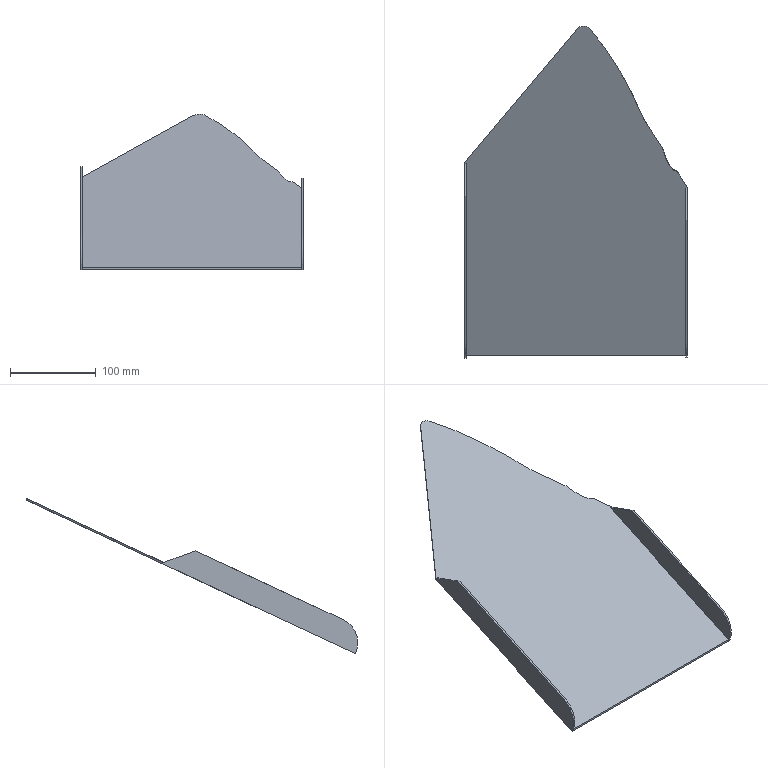Part | NX | features solid 2 | 1 solid | 18 faces | box 260.45 x 387.608 x 181.641 mm | volume 198390 mm3 | plane 12 | spline 3 | cylinder 3 | commonest cylinder face diameters 60 x2 20 x1
STEP:
#1=CARTESIAN_POINT('',(-285.45,-615.955,-192.902));
#2=VERTEX_POINT('',#1);
#3=CARTESIAN_POINT('',(-283.45,-615.955,-192.902));
#4=VERTEX_POINT('',#3);
#5=CARTESIAN_POINT('',(-285.45,-615.955,-192.902));
#6=DIRECTION('',(-1.,0.,0.));
#7=VECTOR('',#6,1000.);
#8=LINE('',#5,#7);
#9=EDGE_CURVE('',#2,#4,#8,.F.);
#10=ORIENTED_EDGE('',*,*,#9,.T.);
#11=CARTESIAN_POINT('',(-283.45,-840.,-297.376));
#12=VERTEX_POINT('',#11);
#13=CARTESIAN_POINT('',(-283.45,-651.161,-209.318));
#14=DIRECTION('',(0.,-0.9063,-0.4226));
#15=VECTOR('',#14,1000.);
#16=LINE('',#13,#15);
#17=EDGE_CURVE('',#4,#12,#16,.T.);
#18=ORIENTED_EDGE('',*,*,#17,.T.);
#19=CARTESIAN_POINT('',(-27.,-840.,-297.376));
#20=VERTEX_POINT('',#19);
#21=CARTESIAN_POINT('',(-1209.175,-840.,-297.376));
#22=DIRECTION('',(-1.,0.,0.));
#23=VECTOR('',#22,1000.);
#24=LINE('',#21,#23);
#25=EDGE_CURVE('',#12,#20,#24,.F.);
#26=ORIENTED_EDGE('',*,*,#25,.T.);
#27=CARTESIAN_POINT('',(-27.,-644.804,-206.354));
#28=VERTEX_POINT('',#27);
#29=CARTESIAN_POINT('',(-27.,-651.161,-209.318));
#30=DIRECTION('',(0.,-0.9063,-0.4226));
#31=VECTOR('',#30,1000.);
#32=LINE('',#29,#31);
#33=EDGE_CURVE('',#28,#20,#32,.T.);
#34=ORIENTED_EDGE('',*,*,#33,.F.);
#35=CARTESIAN_POINT('',(-25.,-644.804,-206.354));
#36=VERTEX_POINT('',#35);
#37=CARTESIAN_POINT('',(-25.,-644.804,-206.354));
#38=DIRECTION('',(1.,0.,0.));
#39=VECTOR('',#38,1000.);
#40=LINE('',#37,#39);
#41=EDGE_CURVE('',#28,#36,#40,.T.);
#42=ORIENTED_EDGE('',*,*,#41,.T.);
#43=CARTESIAN_POINT('',(-25.,-643.958,-205.96));
#44=VERTEX_POINT('',#43);
#45=CARTESIAN_POINT('',(-25.,-651.161,-209.318));
#46=DIRECTION('',(0.,-0.9063,-0.4226));
#47=VECTOR('',#46,1000.);
#48=LINE('',#45,#47);
#49=EDGE_CURVE('',#44,#36,#48,.T.);
#50=ORIENTED_EDGE('',*,*,#49,.F.);
#51=CARTESIAN_POINT('',(-36.874,-625.397,-197.305));
#52=VERTEX_POINT('',#51);
#53=CARTESIAN_POINT('',(-25.,-643.958,-205.96));
#54=CARTESIAN_POINT('',(-28.958,-637.771,-203.075));
#55=CARTESIAN_POINT('',(-32.916,-631.584,-200.19));
#56=CARTESIAN_POINT('',(-36.874,-625.397,-197.305));
#57=B_SPLINE_CURVE_WITH_KNOTS('',3,(#53,#54,#55,#56),.UNSPECIFIED.,.F.,.F.,(4,4),(0.,0.02367),.UNSPECIFIED.);
#58=EDGE_CURVE('',#44,#52,#57,.T.);
#59=ORIENTED_EDGE('',*,*,#58,.T.);
#60=CARTESIAN_POINT('',(-53.995,-598.635,-184.825));
#61=VERTEX_POINT('',#60);
#62=CARTESIAN_POINT('',(-36.874,-625.397,-197.305));
#63=CARTESIAN_POINT('',(-39.726,-624.678,-196.969));
#64=CARTESIAN_POINT('',(-44.629,-621.228,-195.361));
#65=CARTESIAN_POINT('',(-48.688,-613.987,-191.984));
#66=CARTESIAN_POINT('',(-51.509,-606.353,-188.424));
#67=CARTESIAN_POINT('',(-53.147,-601.203,-186.022));
#68=CARTESIAN_POINT('',(-53.995,-598.635,-184.825));
#69=B_SPLINE_CURVE_WITH_KNOTS('',3,(#62,#63,#64,#65,#66,#67,#68),.UNSPECIFIED.,.F.,.F.,(4,1,1,1,4),(0.0119,0.0208,0.0297,0.0386,0.0475),.UNSPECIFIED.);
#70=EDGE_CURVE('',#52,#61,#69,.T.);
#71=ORIENTED_EDGE('',*,*,#70,.T.);
#72=CARTESIAN_POINT('',(-139.243,-458.439,-119.451));
#73=VERTEX_POINT('',#72);
#74=CARTESIAN_POINT('',(-53.995,-598.635,-184.825));
#75=CARTESIAN_POINT('',(-55.837,-595.756,-183.483));
#76=CARTESIAN_POINT('',(-59.52,-589.999,-180.798));
#77=CARTESIAN_POINT('',(-65.043,-581.362,-176.77));
#78=CARTESIAN_POINT('',(-69.653,-574.168,-173.416));
#79=CARTESIAN_POINT('',(-72.866,-569.125,-171.064));
#80=CARTESIAN_POINT('',(-74.724,-566.254,-169.726));
#81=CARTESIAN_POINT('',(-76.066,-564.075,-168.71));
#82=CARTESIAN_POINT('',(-77.109,-561.743,-167.622));
#83=CARTESIAN_POINT('',(-78.457,-559.567,-166.607));
#84=CARTESIAN_POINT('',(-79.554,-557.262,-165.533));
#85=CARTESIAN_POINT('',(-80.855,-554.106,-164.061));
#86=CARTESIAN_POINT('',(-82.504,-550.172,-162.227));
#87=CARTESIAN_POINT('',(-86.598,-540.797,-157.855));
#88=CARTESIAN_POINT('',(-93.303,-527.007,-151.425));
#89=CARTESIAN_POINT('',(-103.21,-509.091,-143.07));
#90=CARTESIAN_POINT('',(-114.016,-491.603,-134.915));
#91=CARTESIAN_POINT('',(-125.687,-474.559,-126.967));
#92=CARTESIAN_POINT('',(-134.482,-463.624,-121.868));
#93=CARTESIAN_POINT('',(-139.243,-458.439,-119.451));
#94=B_SPLINE_CURVE_WITH_KNOTS('',3,(#74,#75,#76,#77,#78,#79,#80,#81,#82,#83,#84,#85,#86,#87,#88,#89,#90,#91,#92,#93),.UNSPECIFIED.,.F.,.F.,(4,1,1,1,1,1,1,1,1,1,1,1,1,1,1,1,1,4),(0.0578,0.06882,0.07983,0.09085,0.09635,0.09911,0.1019,0.1046,0.1074,0.1101,0.1129,0.1184,0.1239,0.1459,0.1679,0.19,0.212,0.234),.UNSPECIFIED.);
#95=EDGE_CURVE('',#61,#73,#94,.T.);
#96=ORIENTED_EDGE('',*,*,#95,.T.);
#97=CARTESIAN_POINT('',(-154.269,-458.775,-119.607));
#98=VERTEX_POINT('',#97);
#99=CARTESIAN_POINT('',(-146.609,-465.203,-122.605));
#100=DIRECTION('',(0.,-0.4226,0.9063));
#101=DIRECTION('',(0.,-0.9063,-0.4226));
#102=AXIS2_PLACEMENT_3D('',#99,#100,#101);
#103=ELLIPSE('',#102,11.034,10.);
#104=EDGE_CURVE('',#73,#98,#103,.T.);
#105=ORIENTED_EDGE('',*,*,#104,.T.);
#106=CARTESIAN_POINT('',(-285.45,-615.11,-192.507));
#107=VERTEX_POINT('',#106);
#108=CARTESIAN_POINT('',(-643.087,-1041.326,-391.255));
#109=DIRECTION('',(0.6053,0.7214,0.3364));
#110=VECTOR('',#109,1000.);
#111=LINE('',#108,#110);
#112=EDGE_CURVE('',#107,#98,#111,.T.);
#113=ORIENTED_EDGE('',*,*,#112,.F.);
#114=CARTESIAN_POINT('',(-285.45,-651.161,-209.318));
#115=DIRECTION('',(0.,-0.9063,-0.4226));
#116=VECTOR('',#115,1000.);
#117=LINE('',#114,#116);
#118=EDGE_CURVE('',#107,#2,#117,.T.);
#119=ORIENTED_EDGE('',*,*,#118,.T.);
#120=EDGE_LOOP('',(#10,#18,#26,#34,#42,#50,#59,#71,#96,#105,#113,#119));
#121=FACE_BOUND('',#120,.T.);
#122=CARTESIAN_POINT('',(-1209.175,-651.161,-209.318));
#123=DIRECTION('',(0.,-0.4226,0.9063));
#124=DIRECTION('',(1.,0.,0.));
#125=AXIS2_PLACEMENT_3D('',#122,#123,#124);
#126=PLANE('',#125);
#127=ADVANCED_FACE('',(#121),#126,.T.);
#128=ORIENTED_EDGE('',*,*,#25,.F.);
#129=CARTESIAN_POINT('',(-283.45,-840.,-299.582));
#130=VERTEX_POINT('',#129);
#131=CARTESIAN_POINT('',(-283.45,-840.,-720.));
#132=DIRECTION('',(0.,0.,1.));
#133=VECTOR('',#132,1000.);
#134=LINE('',#131,#133);
#135=EDGE_CURVE('',#12,#130,#134,.F.);
#136=ORIENTED_EDGE('',*,*,#135,.T.);
#137=CARTESIAN_POINT('',(-27.,-840.,-299.582));
#138=VERTEX_POINT('',#137);
#139=CARTESIAN_POINT('',(-1209.175,-840.,-299.582));
#140=DIRECTION('',(-1.,0.,0.));
#141=VECTOR('',#140,1000.);
#142=LINE('',#139,#141);
#143=EDGE_CURVE('',#130,#138,#142,.F.);
#144=ORIENTED_EDGE('',*,*,#143,.T.);
#145=CARTESIAN_POINT('',(-27.,-840.,-720.));
#146=DIRECTION('',(0.,0.,1.));
#147=VECTOR('',#146,1000.);
#148=LINE('',#145,#147);
#149=EDGE_CURVE('',#20,#138,#148,.F.);
#150=ORIENTED_EDGE('',*,*,#149,.F.);
#151=EDGE_LOOP('',(#128,#136,#144,#150));
#152=FACE_BOUND('',#151,.T.);
#153=CARTESIAN_POINT('',(-476.248,-840.,-720.));
#154=DIRECTION('',(0.,1.,0.));
#155=DIRECTION('',(-1.,0.,0.));
#156=AXIS2_PLACEMENT_3D('',#153,#154,#155);
#157=PLANE('',#156);
#158=ADVANCED_FACE('',(#152),#157,.F.);
#159=CARTESIAN_POINT('',(-285.45,-615.11,-194.714));
#160=VERTEX_POINT('',#159);
#161=CARTESIAN_POINT('',(-285.45,-840.,-299.582));
#162=VERTEX_POINT('',#161);
#163=CARTESIAN_POINT('',(-285.45,-650.315,-211.131));
#164=DIRECTION('',(0.,-0.9063,-0.4226));
#165=VECTOR('',#164,1000.);
#166=LINE('',#163,#165);
#167=EDGE_CURVE('',#160,#162,#166,.T.);
#168=ORIENTED_EDGE('',*,*,#167,.F.);
#169=CARTESIAN_POINT('',(-154.269,-458.775,-121.814));
#170=VERTEX_POINT('',#169);
#171=CARTESIAN_POINT('',(-642.638,-1040.79,-393.212));
#172=DIRECTION('',(0.6053,0.7214,0.3364));
#173=VECTOR('',#172,1000.);
#174=LINE('',#171,#173);
#175=EDGE_CURVE('',#160,#170,#174,.T.);
#176=ORIENTED_EDGE('',*,*,#175,.T.);
#177=CARTESIAN_POINT('',(-139.243,-458.439,-121.657));
#178=VERTEX_POINT('',#177);
#179=CARTESIAN_POINT('',(-146.609,-465.203,-124.811));
#180=DIRECTION('',(0.,-0.4226,0.9063));
#181=DIRECTION('',(0.,-0.9063,-0.4226));
#182=AXIS2_PLACEMENT_3D('',#179,#180,#181);
#183=ELLIPSE('',#182,11.034,10.);
#184=EDGE_CURVE('',#170,#178,#183,.F.);
#185=ORIENTED_EDGE('',*,*,#184,.T.);
#186=CARTESIAN_POINT('',(-53.417,-599.538,-187.453));
#187=VERTEX_POINT('',#186);
#188=CARTESIAN_POINT('',(-53.417,-599.538,-187.453));
#189=CARTESIAN_POINT('',(-55.271,-596.64,-186.102));
#190=CARTESIAN_POINT('',(-58.978,-590.845,-183.399));
#191=CARTESIAN_POINT('',(-64.541,-582.153,-179.346));
#192=CARTESIAN_POINT('',(-69.169,-574.906,-175.967));
#193=CARTESIAN_POINT('',(-72.423,-569.841,-173.605));
#194=CARTESIAN_POINT('',(-74.261,-566.935,-172.25));
#195=CARTESIAN_POINT('',(-75.7,-564.787,-171.248));
#196=CARTESIAN_POINT('',(-76.761,-562.445,-170.156));
#197=CARTESIAN_POINT('',(-78.054,-560.222,-169.12));
#198=CARTESIAN_POINT('',(-79.26,-557.954,-168.062));
#199=CARTESIAN_POINT('',(-80.578,-554.782,-166.583));
#200=CARTESIAN_POINT('',(-82.227,-550.817,-164.734));
#201=CARTESIAN_POINT('',(-86.333,-541.374,-160.331));
#202=CARTESIAN_POINT('',(-93.051,-527.479,-153.852));
#203=CARTESIAN_POINT('',(-103.006,-509.438,-145.439));
#204=CARTESIAN_POINT('',(-113.867,-491.828,-137.227));
#205=CARTESIAN_POINT('',(-125.604,-474.667,-129.225));
#206=CARTESIAN_POINT('',(-134.451,-463.657,-124.091));
#207=CARTESIAN_POINT('',(-139.243,-458.439,-121.657));
#208=B_SPLINE_CURVE_WITH_KNOTS('',3,(#188,#189,#190,#191,#192,#193,#194,#195,#196,#197,#198,#199,#200,#201,#202,#203,#204,#205,#206,#207),.UNSPECIFIED.,.F.,.F.,(4,1,1,1,1,1,1,1,1,1,1,1,1,1,1,1,1,4),(0.05665,0.06774,0.07882,0.08991,0.09545,0.09823,0.101,0.1038,0.1065,0.1093,0.1121,0.1176,0.1232,0.1453,0.1675,0.1897,0.2119,0.234),.UNSPECIFIED.);
#209=EDGE_CURVE('',#187,#178,#208,.T.);
#210=ORIENTED_EDGE('',*,*,#209,.F.);
#211=CARTESIAN_POINT('',(-37.534,-624.366,-199.031));
#212=VERTEX_POINT('',#211);
#213=CARTESIAN_POINT('',(-37.534,-624.366,-199.031));
#214=CARTESIAN_POINT('',(-40.104,-623.568,-198.658));
#215=CARTESIAN_POINT('',(-44.555,-620.328,-197.148));
#216=CARTESIAN_POINT('',(-48.394,-613.718,-194.065));
#217=CARTESIAN_POINT('',(-51.125,-606.69,-190.788));
#218=CARTESIAN_POINT('',(-52.632,-601.916,-188.562));
#219=CARTESIAN_POINT('',(-53.417,-599.538,-187.453));
#220=B_SPLINE_CURVE_WITH_KNOTS('',3,(#213,#214,#215,#216,#217,#218,#219),.UNSPECIFIED.,.F.,.F.,(4,1,1,1,4),(0.0126,0.02081,0.02901,0.03722,0.04543),.UNSPECIFIED.);
#221=EDGE_CURVE('',#212,#187,#220,.T.);
#222=ORIENTED_EDGE('',*,*,#221,.F.);
#223=CARTESIAN_POINT('',(-25.,-643.958,-208.167));
#224=VERTEX_POINT('',#223);
#225=CARTESIAN_POINT('',(-25.,-643.958,-208.167));
#226=CARTESIAN_POINT('',(-29.178,-637.428,-205.121));
#227=CARTESIAN_POINT('',(-33.356,-630.897,-202.076));
#228=CARTESIAN_POINT('',(-37.534,-624.366,-199.031));
#229=B_SPLINE_CURVE_WITH_KNOTS('',3,(#225,#226,#227,#228),.UNSPECIFIED.,.F.,.F.,(4,4),(0.,0.02499),.UNSPECIFIED.);
#230=EDGE_CURVE('',#224,#212,#229,.T.);
#231=ORIENTED_EDGE('',*,*,#230,.F.);
#232=CARTESIAN_POINT('',(-25.,-840.,-299.582));
#233=VERTEX_POINT('',#232);
#234=CARTESIAN_POINT('',(-25.,-650.315,-211.131));
#235=DIRECTION('',(0.,-0.9063,-0.4226));
#236=VECTOR('',#235,1000.);
#237=LINE('',#234,#236);
#238=EDGE_CURVE('',#224,#233,#237,.T.);
#239=ORIENTED_EDGE('',*,*,#238,.T.);
#240=CARTESIAN_POINT('',(-25.,-840.,-299.582));
#241=DIRECTION('',(1.,0.,0.));
#242=VECTOR('',#241,1000.);
#243=LINE('',#240,#242);
#244=EDGE_CURVE('',#233,#138,#243,.F.);
#245=ORIENTED_EDGE('',*,*,#244,.T.);
#246=ORIENTED_EDGE('',*,*,#143,.F.);
#247=CARTESIAN_POINT('',(-1209.175,-840.,-299.582));
#248=DIRECTION('',(-1.,0.,0.));
#249=VECTOR('',#248,1000.);
#250=LINE('',#247,#249);
#251=EDGE_CURVE('',#162,#130,#250,.F.);
#252=ORIENTED_EDGE('',*,*,#251,.F.);
#253=EDGE_LOOP('',(#168,#176,#185,#210,#222,#231,#239,#245,#246,#252));
#254=FACE_BOUND('',#253,.T.);
#255=CARTESIAN_POINT('',(-1209.175,-650.315,-211.131));
#256=DIRECTION('',(0.,-0.4226,0.9063));
#257=DIRECTION('',(1.,0.,0.));
#258=AXIS2_PLACEMENT_3D('',#255,#256,#257);
#259=PLANE('',#258);
#260=ADVANCED_FACE('',(#254),#259,.F.);
#261=ORIENTED_EDGE('',*,*,#238,.F.);
#262=CARTESIAN_POINT('',(-25.,-643.958,-172.786));
#263=DIRECTION('',(0.,0.,-1.));
#264=VECTOR('',#263,1000.);
#265=LINE('',#262,#264);
#266=EDGE_CURVE('',#224,#44,#265,.F.);
#267=ORIENTED_EDGE('',*,*,#266,.T.);
#268=ORIENTED_EDGE('',*,*,#49,.T.);
#269=CARTESIAN_POINT('',(-25.,-682.014,-192.811));
#270=VERTEX_POINT('',#269);
#271=CARTESIAN_POINT('',(-25.,-682.014,-192.811));
#272=DIRECTION('',(0.,0.9397,-0.342));
#273=VECTOR('',#272,1000.);
#274=LINE('',#271,#273);
#275=EDGE_CURVE('',#36,#270,#274,.F.);
#276=ORIENTED_EDGE('',*,*,#275,.T.);
#277=CARTESIAN_POINT('',(-25.,-825.489,-259.715));
#278=VERTEX_POINT('',#277);
#279=CARTESIAN_POINT('',(-25.,-656.637,-180.977));
#280=DIRECTION('',(0.,-0.9063,-0.4226));
#281=VECTOR('',#280,1000.);
#282=LINE('',#279,#281);
#283=EDGE_CURVE('',#270,#278,#282,.T.);
#284=ORIENTED_EDGE('',*,*,#283,.T.);
#285=CARTESIAN_POINT('',(-25.,-812.811,-286.904));
#286=DIRECTION('',(-1.,0.,0.));
#287=DIRECTION('',(0.,-1.,0.));
#288=AXIS2_PLACEMENT_3D('',#285,#286,#287);
#289=CIRCLE('',#288,30.);
#290=EDGE_CURVE('',#278,#233,#289,.F.);
#291=ORIENTED_EDGE('',*,*,#290,.T.);
#292=EDGE_LOOP('',(#261,#267,#268,#276,#284,#291));
#293=FACE_BOUND('',#292,.T.);
#294=CARTESIAN_POINT('',(-25.,-651.161,-209.318));
#295=DIRECTION('',(1.,0.,0.));
#296=DIRECTION('',(0.,1.,0.));
#297=AXIS2_PLACEMENT_3D('',#294,#295,#296);
#298=PLANE('',#297);
#299=ADVANCED_FACE('',(#293),#298,.T.);
#300=CARTESIAN_POINT('',(-53.995,-598.635,-184.825));
#301=CARTESIAN_POINT('',(-53.802,-598.936,-185.701));
#302=CARTESIAN_POINT('',(-53.61,-599.237,-186.577));
#303=CARTESIAN_POINT('',(-53.417,-599.538,-187.453));
#304=B_SPLINE_CURVE_WITH_KNOTS('',3,(#300,#301,#302,#303),.UNSPECIFIED.,.F.,.F.,(4,4),(0.,0.002838),.UNSPECIFIED.);
#305=EDGE_CURVE('',#61,#187,#304,.T.);
#306=ORIENTED_EDGE('',*,*,#305,.F.);
#307=ORIENTED_EDGE('',*,*,#70,.F.);
#308=CARTESIAN_POINT('',(-37.534,-624.366,-199.031));
#309=CARTESIAN_POINT('',(-37.309,-624.717,-198.461));
#310=CARTESIAN_POINT('',(-37.09,-625.06,-197.885));
#311=CARTESIAN_POINT('',(-36.874,-625.397,-197.305));
#312=B_SPLINE_CURVE_WITH_KNOTS('',3,(#308,#309,#310,#311),.UNSPECIFIED.,.F.,.F.,(4,4),(0.,0.002116),.UNSPECIFIED.);
#313=EDGE_CURVE('',#212,#52,#312,.T.);
#314=ORIENTED_EDGE('',*,*,#313,.F.);
#315=ORIENTED_EDGE('',*,*,#221,.T.);
#316=EDGE_LOOP('',(#306,#307,#314,#315));
#317=FACE_BOUND('',#316,.T.);
#318=CARTESIAN_POINT('',(-36.683,-625.444,-197.326));
#319=CARTESIAN_POINT('',(-36.683,-624.599,-199.139));
#320=CARTESIAN_POINT('',(-38.04,-625.123,-197.177));
#321=CARTESIAN_POINT('',(-38.04,-624.278,-198.989));
#322=CARTESIAN_POINT('',(-39.942,-624.34,-196.811));
#323=CARTESIAN_POINT('',(-39.942,-623.494,-198.624));
#324=CARTESIAN_POINT('',(-42.329,-622.626,-196.012));
#325=CARTESIAN_POINT('',(-42.329,-621.78,-197.825));
#326=CARTESIAN_POINT('',(-43.737,-621.301,-195.395));
#327=CARTESIAN_POINT('',(-43.737,-620.456,-197.207));
#328=CARTESIAN_POINT('',(-44.755,-620.127,-194.847));
#329=CARTESIAN_POINT('',(-44.755,-619.282,-196.66));
#330=CARTESIAN_POINT('',(-45.441,-619.212,-194.42));
#331=CARTESIAN_POINT('',(-45.441,-618.366,-196.233));
#332=CARTESIAN_POINT('',(-45.78,-618.737,-194.199));
#333=CARTESIAN_POINT('',(-45.78,-617.892,-196.012));
#334=CARTESIAN_POINT('',(-46.399,-617.818,-193.77));
#335=CARTESIAN_POINT('',(-46.399,-616.973,-195.583));
#336=CARTESIAN_POINT('',(-47.088,-616.659,-193.23));
#337=CARTESIAN_POINT('',(-47.088,-615.814,-195.043));
#338=CARTESIAN_POINT('',(-47.668,-615.577,-192.725));
#339=CARTESIAN_POINT('',(-47.668,-614.732,-194.538));
#340=CARTESIAN_POINT('',(-48.022,-614.877,-192.399));
#341=CARTESIAN_POINT('',(-48.022,-614.032,-194.212));
#342=CARTESIAN_POINT('',(-48.242,-614.43,-192.19));
#343=CARTESIAN_POINT('',(-48.242,-613.585,-194.003));
#344=CARTESIAN_POINT('',(-48.562,-613.756,-191.876));
#345=CARTESIAN_POINT('',(-48.562,-612.911,-193.689));
#346=CARTESIAN_POINT('',(-49.049,-612.679,-191.374));
#347=CARTESIAN_POINT('',(-49.049,-611.834,-193.187));
#348=CARTESIAN_POINT('',(-49.912,-610.64,-190.423));
#349=CARTESIAN_POINT('',(-49.912,-609.795,-192.236));
#350=CARTESIAN_POINT('',(-51.134,-607.357,-188.892));
#351=CARTESIAN_POINT('',(-51.134,-606.511,-190.705));
#352=CARTESIAN_POINT('',(-52.599,-602.84,-186.786));
#353=CARTESIAN_POINT('',(-52.599,-601.995,-188.599));
#354=CARTESIAN_POINT('',(-53.576,-599.903,-185.416));
#355=CARTESIAN_POINT('',(-53.576,-599.057,-187.229));
#356=CARTESIAN_POINT('',(-54.064,-598.425,-184.727));
#357=CARTESIAN_POINT('',(-54.064,-597.579,-186.54));
#358=B_SPLINE_SURFACE_WITH_KNOTS('',3,1,((#318,#319),(#320,#321),(#322,#323),(#324,#325),(#326,#327),(#328,#329),(#330,#331),(#332,#333),(#334,#335),(#336,#337),(#338,#339),(#340,#341),(#342,#343),(#344,#345),(#346,#347),(#348,#349),(#350,#351),(#352,#353),(#354,#355),(#356,#357)),.SURF_OF_LINEAR_EXTRUSION.,.F.,.F.,.F.,(4,1,1,1,1,1,1,1,1,1,1,1,1,1,1,1,1,4),(2,2),(0.3569,0.4586,0.5094,0.5602,0.611,0.6238,0.6365,0.6619,0.7127,0.7381,0.7508,0.7635,0.7889,0.8143,0.8652,0.9668,1.068,1.17),(0.,1.),.UNSPECIFIED.);
#359=ADVANCED_FACE('',(#317),#358,.F.);
#360=ORIENTED_EDGE('',*,*,#112,.T.);
#361=CARTESIAN_POINT('',(-154.269,-458.775,-117.859));
#362=DIRECTION('',(0.,0.,1.));
#363=VECTOR('',#362,1000.);
#364=LINE('',#361,#363);
#365=EDGE_CURVE('',#98,#170,#364,.F.);
#366=ORIENTED_EDGE('',*,*,#365,.T.);
#367=ORIENTED_EDGE('',*,*,#175,.F.);
#368=CARTESIAN_POINT('',(-285.45,-615.11,-43.214));
#369=DIRECTION('',(0.,0.,1.));
#370=VECTOR('',#369,1000.);
#371=LINE('',#368,#370);
#372=EDGE_CURVE('',#160,#107,#371,.T.);
#373=ORIENTED_EDGE('',*,*,#372,.T.);
#374=EDGE_LOOP('',(#360,#366,#367,#373));
#375=FACE_BOUND('',#374,.T.);
#376=CARTESIAN_POINT('',(-270.418,-597.195,-180.));
#377=DIRECTION('',(0.766,-0.6428,0.));
#378=DIRECTION('',(0.6428,0.766,0.));
#379=AXIS2_PLACEMENT_3D('',#376,#377,#378);
#380=PLANE('',#379);
#381=ADVANCED_FACE('',(#375),#380,.F.);
#382=ORIENTED_EDGE('',*,*,#372,.F.);
#383=ORIENTED_EDGE('',*,*,#167,.T.);
#384=CARTESIAN_POINT('',(-285.45,-825.489,-259.715));
#385=VERTEX_POINT('',#384);
#386=CARTESIAN_POINT('',(-285.45,-812.811,-286.904));
#387=DIRECTION('',(-1.,0.,0.));
#388=DIRECTION('',(0.,-1.,0.));
#389=AXIS2_PLACEMENT_3D('',#386,#387,#388);
#390=CIRCLE('',#389,30.);
#391=EDGE_CURVE('',#162,#385,#390,.T.);
#392=ORIENTED_EDGE('',*,*,#391,.T.);
#393=CARTESIAN_POINT('',(-285.45,-653.165,-179.358));
#394=VERTEX_POINT('',#393);
#395=CARTESIAN_POINT('',(-285.45,-627.788,-167.525));
#396=DIRECTION('',(0.,-0.9063,-0.4226));
#397=VECTOR('',#396,1000.);
#398=LINE('',#395,#397);
#399=EDGE_CURVE('',#394,#385,#398,.T.);
#400=ORIENTED_EDGE('',*,*,#399,.F.);
#401=CARTESIAN_POINT('',(-285.45,-614.626,-193.385));
#402=DIRECTION('',(0.,-0.9397,0.342));
#403=VECTOR('',#402,1000.);
#404=LINE('',#401,#403);
#405=EDGE_CURVE('',#394,#2,#404,.F.);
#406=ORIENTED_EDGE('',*,*,#405,.T.);
#407=ORIENTED_EDGE('',*,*,#118,.F.);
#408=EDGE_LOOP('',(#382,#383,#392,#400,#406,#407));
#409=FACE_BOUND('',#408,.T.);
#410=CARTESIAN_POINT('',(-285.45,-599.053,-43.214));
#411=DIRECTION('',(-1.,0.,0.));
#412=DIRECTION('',(0.,-1.,0.));
#413=AXIS2_PLACEMENT_3D('',#410,#411,#412);
#414=PLANE('',#413);
#415=ADVANCED_FACE('',(#409),#414,.T.);
#416=ORIENTED_EDGE('',*,*,#209,.T.);
#417=CARTESIAN_POINT('',(-139.243,-458.439,-121.657));
#418=DIRECTION('',(0.,0.,-1.));
#419=VECTOR('',#418,1000.);
#420=LINE('',#417,#419);
#421=EDGE_CURVE('',#178,#73,#420,.F.);
#422=ORIENTED_EDGE('',*,*,#421,.T.);
#423=ORIENTED_EDGE('',*,*,#95,.F.);
#424=ORIENTED_EDGE('',*,*,#305,.T.);
#425=EDGE_LOOP('',(#416,#422,#423,#424));
#426=FACE_BOUND('',#425,.T.);
#427=CARTESIAN_POINT('',(-139.243,-458.439,-119.336));
#428=CARTESIAN_POINT('',(-139.243,-458.439,-138.648));
#429=CARTESIAN_POINT('',(-137.11,-460.762,-119.998));
#430=CARTESIAN_POINT('',(-137.11,-460.762,-139.31));
#431=CARTESIAN_POINT('',(-135.039,-463.151,-120.603));
#432=CARTESIAN_POINT('',(-135.039,-463.151,-139.915));
#433=CARTESIAN_POINT('',(-128.569,-470.991,-122.443));
#434=CARTESIAN_POINT('',(-128.569,-470.991,-141.755));
#435=CARTESIAN_POINT('',(-124.405,-476.629,-123.57));
#436=CARTESIAN_POINT('',(-124.405,-476.629,-142.882));
#437=CARTESIAN_POINT('',(-112.544,-493.728,-127.342));
#438=CARTESIAN_POINT('',(-112.544,-493.728,-146.654));
#439=CARTESIAN_POINT('',(-105.346,-505.382,-130.606));
#440=CARTESIAN_POINT('',(-105.346,-505.382,-149.918));
#441=CARTESIAN_POINT('',(-95.589,-522.951,-136.978));
#442=CARTESIAN_POINT('',(-95.589,-522.951,-156.29));
#443=CARTESIAN_POINT('',(-92.511,-528.802,-139.353));
#444=CARTESIAN_POINT('',(-92.511,-528.802,-158.665));
#445=CARTESIAN_POINT('',(-86.771,-540.468,-144.777));
#446=CARTESIAN_POINT('',(-86.771,-540.468,-164.089));
#447=CARTESIAN_POINT('',(-84.158,-546.285,-147.829));
#448=CARTESIAN_POINT('',(-84.158,-546.285,-167.142));
#449=CARTESIAN_POINT('',(-81.188,-553.302,-152.163));
#450=CARTESIAN_POINT('',(-81.188,-553.302,-171.475));
#451=CARTESIAN_POINT('',(-80.613,-554.707,-153.052));
#452=CARTESIAN_POINT('',(-80.613,-554.707,-172.365));
#453=CARTESIAN_POINT('',(-79.478,-557.413,-154.829));
#454=CARTESIAN_POINT('',(-79.478,-557.413,-174.141));
#455=CARTESIAN_POINT('',(-78.981,-558.514,-155.728));
#456=CARTESIAN_POINT('',(-78.981,-558.514,-175.041));
#457=CARTESIAN_POINT('',(-78.3,-559.755,-156.764));
#458=CARTESIAN_POINT('',(-78.3,-559.755,-176.077));
#459=CARTESIAN_POINT('',(-78.224,-559.892,-156.88));
#460=CARTESIAN_POINT('',(-78.224,-559.892,-176.192));
#461=CARTESIAN_POINT('',(-78.068,-560.165,-157.111));
#462=CARTESIAN_POINT('',(-78.068,-560.165,-176.424));
#463=CARTESIAN_POINT('',(-78.006,-560.272,-157.227));
#464=CARTESIAN_POINT('',(-78.006,-560.272,-176.54));
#465=CARTESIAN_POINT('',(-77.691,-560.808,-157.576));
#466=CARTESIAN_POINT('',(-77.691,-560.808,-176.888));
#467=CARTESIAN_POINT('',(-77.495,-561.151,-157.809));
#468=CARTESIAN_POINT('',(-77.495,-561.151,-177.121));
#469=CARTESIAN_POINT('',(-77.069,-561.932,-158.276));
#470=CARTESIAN_POINT('',(-77.069,-561.932,-177.588));
#471=CARTESIAN_POINT('',(-76.871,-562.32,-158.51));
#472=CARTESIAN_POINT('',(-76.871,-562.32,-177.823));
#473=CARTESIAN_POINT('',(-76.502,-563.062,-158.976));
#474=CARTESIAN_POINT('',(-76.502,-563.062,-178.288));
#475=CARTESIAN_POINT('',(-76.354,-563.37,-159.207));
#476=CARTESIAN_POINT('',(-76.354,-563.37,-178.519));
#477=CARTESIAN_POINT('',(-76.039,-564.008,-159.663));
#478=CARTESIAN_POINT('',(-76.039,-564.008,-178.975));
#479=CARTESIAN_POINT('',(-75.92,-564.242,-159.888));
#480=CARTESIAN_POINT('',(-75.92,-564.242,-179.2));
#481=CARTESIAN_POINT('',(-75.639,-564.757,-160.331));
#482=CARTESIAN_POINT('',(-75.639,-564.757,-179.643));
#483=CARTESIAN_POINT('',(-75.493,-565.008,-160.549));
#484=CARTESIAN_POINT('',(-75.493,-565.008,-179.861));
#485=CARTESIAN_POINT('',(-75.015,-565.792,-161.189));
#486=CARTESIAN_POINT('',(-75.015,-565.792,-180.501));
#487=CARTESIAN_POINT('',(-74.576,-566.464,-161.6));
#488=CARTESIAN_POINT('',(-74.576,-566.464,-180.912));
#489=CARTESIAN_POINT('',(-70.878,-572.245,-165.351));
#490=CARTESIAN_POINT('',(-70.878,-572.245,-184.663));
#491=CARTESIAN_POINT('',(-67.59,-577.383,-168.685));
#492=CARTESIAN_POINT('',(-67.59,-577.383,-187.997));
#493=CARTESIAN_POINT('',(-60.506,-588.457,-175.871));
#494=CARTESIAN_POINT('',(-60.506,-588.457,-195.184));
#495=CARTESIAN_POINT('',(-56.709,-594.393,-179.723));
#496=CARTESIAN_POINT('',(-56.709,-594.393,-199.036));
#497=CARTESIAN_POINT('',(-52.911,-600.329,-183.575));
#498=CARTESIAN_POINT('',(-52.911,-600.329,-202.887));
#499=B_SPLINE_SURFACE_WITH_KNOTS('',3,1,((#427,#428),(#429,#430),(#431,#432),(#433,#434),(#435,#436),(#437,#438),(#439,#440),(#441,#442),(#443,#444),(#445,#446),(#447,#448),(#449,#450),(#451,#452),(#453,#454),(#455,#456),(#457,#458),(#459,#460),(#461,#462),(#463,#464),(#465,#466),(#467,#468),(#469,#470),(#471,#472),(#473,#474),(#475,#476),(#477,#478),(#479,#480),(#481,#482),(#483,#484),(#485,#486),(#487,#488),(#489,#490),(#491,#492),(#493,#494),(#495,#496),(#497,#498)),.SURF_OF_LINEAR_EXTRUSION.,.F.,.F.,.F.,(4,2,2,2,2,2,2,2,2,2,2,2,2,2,2,2,2,4),(2,2),(0.3147,0.3389,0.3926,0.5,0.5537,0.6074,0.6208,0.6342,0.6359,0.6376,0.641,0.6443,0.6477,0.651,0.6544,0.6611,0.7148,0.7768),(0.5811,0.6211),.UNSPECIFIED.);
#500=ADVANCED_FACE('',(#426),#499,.T.);
#501=ORIENTED_EDGE('',*,*,#266,.F.);
#502=ORIENTED_EDGE('',*,*,#230,.T.);
#503=ORIENTED_EDGE('',*,*,#313,.T.);
#504=ORIENTED_EDGE('',*,*,#58,.F.);
#505=EDGE_LOOP('',(#501,#502,#503,#504));
#506=FACE_BOUND('',#505,.T.);
#507=CARTESIAN_POINT('',(-37.609,-624.249,-193.135));
#508=CARTESIAN_POINT('',(-37.609,-624.249,-198.989));
#509=CARTESIAN_POINT('',(-33.406,-630.819,-197.399));
#510=CARTESIAN_POINT('',(-33.406,-630.819,-203.252));
#511=CARTESIAN_POINT('',(-29.203,-637.389,-201.662));
#512=CARTESIAN_POINT('',(-29.203,-637.389,-207.516));
#513=CARTESIAN_POINT('',(-25.,-643.958,-205.925));
#514=CARTESIAN_POINT('',(-25.,-643.958,-211.779));
#515=B_SPLINE_SURFACE_WITH_KNOTS('',3,1,((#507,#508),(#509,#510),(#511,#512),(#513,#514)),.SURF_OF_LINEAR_EXTRUSION.,.F.,.F.,.F.,(4,4),(2,2),(0.8602,0.9288),(0.5687,0.5808),.PIECEWISE_BEZIER_KNOTS.);
#516=ADVANCED_FACE('',(#506),#515,.T.);
#517=ORIENTED_EDGE('',*,*,#184,.F.);
#518=ORIENTED_EDGE('',*,*,#365,.F.);
#519=ORIENTED_EDGE('',*,*,#104,.F.);
#520=ORIENTED_EDGE('',*,*,#421,.F.);
#521=EDGE_LOOP('',(#517,#518,#519,#520));
#522=FACE_BOUND('',#521,.T.);
#523=CARTESIAN_POINT('',(-146.609,-465.203,-116.755));
#524=DIRECTION('',(0.,0.,-1.));
#525=DIRECTION('',(-1.,0.,0.));
#526=AXIS2_PLACEMENT_3D('',#523,#524,#525);
#527=CYLINDRICAL_SURFACE('',#526,10.);
#528=ADVANCED_FACE('',(#522),#527,.T.);
#529=ORIENTED_EDGE('',*,*,#283,.F.);
#530=CARTESIAN_POINT('',(-27.,-682.014,-192.811));
#531=VERTEX_POINT('',#530);
#532=CARTESIAN_POINT('',(-25.,-682.014,-192.811));
#533=DIRECTION('',(-1.,0.,0.));
#534=VECTOR('',#533,1000.);
#535=LINE('',#532,#534);
#536=EDGE_CURVE('',#270,#531,#535,.T.);
#537=ORIENTED_EDGE('',*,*,#536,.T.);
#538=CARTESIAN_POINT('',(-27.,-825.489,-259.715));
#539=VERTEX_POINT('',#538);
#540=CARTESIAN_POINT('',(-27.,-656.637,-180.977));
#541=DIRECTION('',(0.,-0.9063,-0.4226));
#542=VECTOR('',#541,1000.);
#543=LINE('',#540,#542);
#544=EDGE_CURVE('',#531,#539,#543,.T.);
#545=ORIENTED_EDGE('',*,*,#544,.T.);
#546=CARTESIAN_POINT('',(-25.,-825.489,-259.715));
#547=DIRECTION('',(1.,0.,0.));
#548=VECTOR('',#547,1000.);
#549=LINE('',#546,#548);
#550=EDGE_CURVE('',#539,#278,#549,.T.);
#551=ORIENTED_EDGE('',*,*,#550,.T.);
#552=EDGE_LOOP('',(#529,#537,#545,#551));
#553=FACE_BOUND('',#552,.T.);
#554=CARTESIAN_POINT('',(-25.,-656.637,-180.977));
#555=DIRECTION('',(0.,0.4226,-0.9063));
#556=DIRECTION('',(0.,-0.9063,-0.4226));
#557=AXIS2_PLACEMENT_3D('',#554,#555,#556);
#558=PLANE('',#557);
#559=ADVANCED_FACE('',(#553),#558,.F.);
#560=CARTESIAN_POINT('',(-27.,-643.475,-206.838));
#561=DIRECTION('',(0.,-0.9397,0.342));
#562=VECTOR('',#561,1000.);
#563=LINE('',#560,#562);
#564=EDGE_CURVE('',#531,#28,#563,.F.);
#565=ORIENTED_EDGE('',*,*,#564,.T.);
#566=ORIENTED_EDGE('',*,*,#33,.T.);
#567=ORIENTED_EDGE('',*,*,#149,.T.);
#568=CARTESIAN_POINT('',(-27.,-812.811,-286.904));
#569=DIRECTION('',(-1.,0.,0.));
#570=DIRECTION('',(0.,-1.,0.));
#571=AXIS2_PLACEMENT_3D('',#568,#569,#570);
#572=CIRCLE('',#571,30.);
#573=EDGE_CURVE('',#138,#539,#572,.T.);
#574=ORIENTED_EDGE('',*,*,#573,.T.);
#575=ORIENTED_EDGE('',*,*,#544,.F.);
#576=EDGE_LOOP('',(#565,#566,#567,#574,#575));
#577=FACE_BOUND('',#576,.T.);
#578=CARTESIAN_POINT('',(-27.,-643.958,-208.167));
#579=DIRECTION('',(-1.,0.,0.));
#580=DIRECTION('',(0.,-1.,0.));
#581=AXIS2_PLACEMENT_3D('',#578,#579,#580);
#582=PLANE('',#581);
#583=ADVANCED_FACE('',(#577),#582,.T.);
#584=ORIENTED_EDGE('',*,*,#290,.F.);
#585=ORIENTED_EDGE('',*,*,#550,.F.);
#586=ORIENTED_EDGE('',*,*,#573,.F.);
#587=ORIENTED_EDGE('',*,*,#244,.F.);
#588=EDGE_LOOP('',(#584,#585,#586,#587));
#589=FACE_BOUND('',#588,.T.);
#590=CARTESIAN_POINT('',(-25.,-812.811,-286.904));
#591=DIRECTION('',(1.,0.,0.));
#592=DIRECTION('',(0.,1.,0.));
#593=AXIS2_PLACEMENT_3D('',#590,#591,#592);
#594=CYLINDRICAL_SURFACE('',#593,30.);
#595=ADVANCED_FACE('',(#589),#594,.T.);
#596=ORIENTED_EDGE('',*,*,#275,.F.);
#597=ORIENTED_EDGE('',*,*,#41,.F.);
#598=ORIENTED_EDGE('',*,*,#564,.F.);
#599=ORIENTED_EDGE('',*,*,#536,.F.);
#600=EDGE_LOOP('',(#596,#597,#598,#599));
#601=FACE_BOUND('',#600,.T.);
#602=CARTESIAN_POINT('',(-25.,-682.014,-192.811));
#603=DIRECTION('',(0.,-0.342,-0.9397));
#604=DIRECTION('',(0.,0.9397,-0.342));
#605=AXIS2_PLACEMENT_3D('',#602,#603,#604);
#606=PLANE('',#605);
#607=ADVANCED_FACE('',(#601),#606,.F.);
#608=CARTESIAN_POINT('',(-283.45,-653.165,-179.358));
#609=VERTEX_POINT('',#608);
#610=CARTESIAN_POINT('',(-283.45,-825.489,-259.715));
#611=VERTEX_POINT('',#610);
#612=CARTESIAN_POINT('',(-283.45,-627.788,-167.525));
#613=DIRECTION('',(0.,-0.9063,-0.4226));
#614=VECTOR('',#613,1000.);
#615=LINE('',#612,#614);
#616=EDGE_CURVE('',#609,#611,#615,.T.);
#617=ORIENTED_EDGE('',*,*,#616,.F.);
#618=CARTESIAN_POINT('',(-285.45,-653.165,-179.358));
#619=DIRECTION('',(1.,0.,0.));
#620=VECTOR('',#619,1000.);
#621=LINE('',#618,#620);
#622=EDGE_CURVE('',#609,#394,#621,.F.);
#623=ORIENTED_EDGE('',*,*,#622,.T.);
#624=ORIENTED_EDGE('',*,*,#399,.T.);
#625=CARTESIAN_POINT('',(-285.45,-825.489,-259.715));
#626=DIRECTION('',(1.,0.,0.));
#627=VECTOR('',#626,1000.);
#628=LINE('',#625,#627);
#629=EDGE_CURVE('',#385,#611,#628,.T.);
#630=ORIENTED_EDGE('',*,*,#629,.T.);
#631=EDGE_LOOP('',(#617,#623,#624,#630));
#632=FACE_BOUND('',#631,.T.);
#633=CARTESIAN_POINT('',(-285.45,-627.788,-167.525));
#634=DIRECTION('',(0.,0.4226,-0.9063));
#635=DIRECTION('',(0.,-0.9063,-0.4226));
#636=AXIS2_PLACEMENT_3D('',#633,#634,#635);
#637=PLANE('',#636);
#638=ADVANCED_FACE('',(#632),#637,.F.);
#639=ORIENTED_EDGE('',*,*,#17,.F.);
#640=CARTESIAN_POINT('',(-283.45,-615.955,-192.902));
#641=DIRECTION('',(0.,0.9397,-0.342));
#642=VECTOR('',#641,1000.);
#643=LINE('',#640,#642);
#644=EDGE_CURVE('',#4,#609,#643,.F.);
#645=ORIENTED_EDGE('',*,*,#644,.T.);
#646=ORIENTED_EDGE('',*,*,#616,.T.);
#647=CARTESIAN_POINT('',(-283.45,-812.811,-286.904));
#648=DIRECTION('',(-1.,0.,0.));
#649=DIRECTION('',(0.,-1.,0.));
#650=AXIS2_PLACEMENT_3D('',#647,#648,#649);
#651=CIRCLE('',#650,30.);
#652=EDGE_CURVE('',#611,#130,#651,.F.);
#653=ORIENTED_EDGE('',*,*,#652,.T.);
#654=ORIENTED_EDGE('',*,*,#135,.F.);
#655=EDGE_LOOP('',(#639,#645,#646,#653,#654));
#656=FACE_BOUND('',#655,.T.);
#657=CARTESIAN_POINT('',(-283.45,-615.11,-194.714));
#658=DIRECTION('',(-1.,0.,0.));
#659=DIRECTION('',(0.,-1.,0.));
#660=AXIS2_PLACEMENT_3D('',#657,#658,#659);
#661=PLANE('',#660);
#662=ADVANCED_FACE('',(#656),#661,.F.);
#663=ORIENTED_EDGE('',*,*,#391,.F.);
#664=ORIENTED_EDGE('',*,*,#251,.T.);
#665=ORIENTED_EDGE('',*,*,#652,.F.);
#666=ORIENTED_EDGE('',*,*,#629,.F.);
#667=EDGE_LOOP('',(#663,#664,#665,#666));
#668=FACE_BOUND('',#667,.T.);
#669=CARTESIAN_POINT('',(-285.45,-812.811,-286.904));
#670=DIRECTION('',(-1.,0.,0.));
#671=DIRECTION('',(0.,-1.,0.));
#672=AXIS2_PLACEMENT_3D('',#669,#670,#671);
#673=CYLINDRICAL_SURFACE('',#672,30.);
#674=ADVANCED_FACE('',(#668),#673,.T.);
#675=ORIENTED_EDGE('',*,*,#405,.F.);
#676=ORIENTED_EDGE('',*,*,#622,.F.);
#677=ORIENTED_EDGE('',*,*,#644,.F.);
#678=ORIENTED_EDGE('',*,*,#9,.F.);
#679=EDGE_LOOP('',(#675,#676,#677,#678));
#680=FACE_BOUND('',#679,.T.);
#681=CARTESIAN_POINT('',(-285.45,-615.955,-192.902));
#682=DIRECTION('',(0.,-0.342,-0.9397));
#683=DIRECTION('',(0.,0.9397,-0.342));
#684=AXIS2_PLACEMENT_3D('',#681,#682,#683);
#685=PLANE('',#684);
#686=ADVANCED_FACE('',(#680),#685,.F.);
#687=CLOSED_SHELL('',(#127,#158,#260,#299,#359,#381,#415,#500,#516,#528,#559,#583,#595,#607,#638,#662,#674,#686));
#688=MANIFOLD_SOLID_BREP('',#687);
#689=(LENGTH_UNIT()NAMED_UNIT(*)SI_UNIT(.MILLI.,.METRE.));
#690=UNCERTAINTY_MEASURE_WITH_UNIT(LENGTH_MEASURE(0.0508),#689,'','');
#691=(NAMED_UNIT(*)PLANE_ANGLE_UNIT()SI_UNIT($,.RADIAN.));
#692=(NAMED_UNIT(*)SI_UNIT($,.STERADIAN.)SOLID_ANGLE_UNIT());
#693=(GEOMETRIC_REPRESENTATION_CONTEXT(3)GLOBAL_UNCERTAINTY_ASSIGNED_CONTEXT((#690))GLOBAL_UNIT_ASSIGNED_CONTEXT((#689,#691,#692))REPRESENTATION_CONTEXT('',''));
#694=ADVANCED_BREP_SHAPE_REPRESENTATION('',(#688),#693);